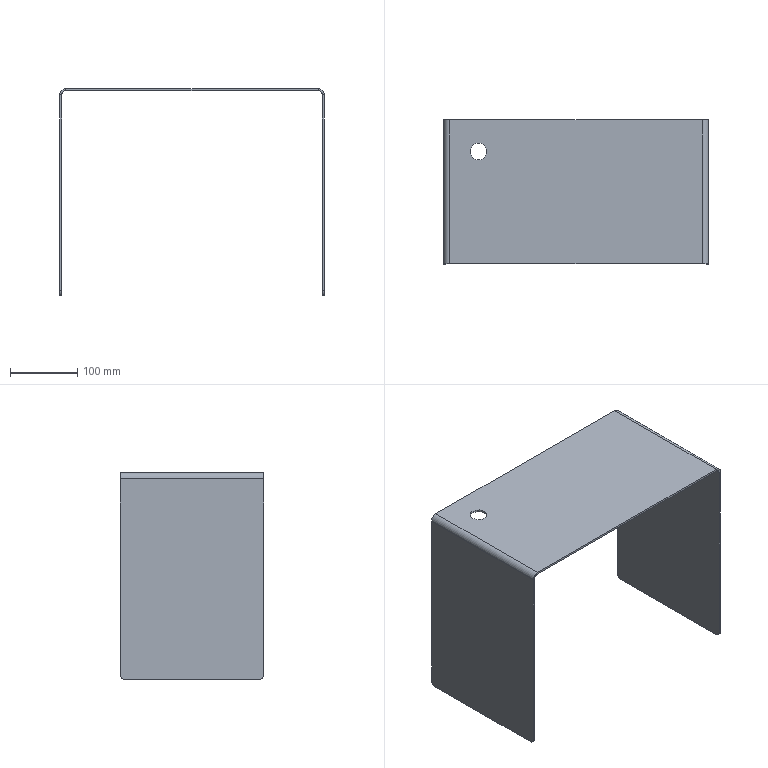Part | SolidWorks | features Fillet 1, FlatPattern 1, ICE 1, SMBaseFlange 1, SheetMetal 1 | 1 solid | 28 faces | box 394 x 214 x 307 mm | volume 637569 mm3 | plane 18 | cylinder 10 | commonest cylinder face diameters 13 x4 12 x2 18 x2 25 x2
STEP:
#1=CARTESIAN_POINT('',(64.5,167.,0.));
#2=VERTEX_POINT('',#1);
#3=CARTESIAN_POINT('',(39.5,167.,0.));
#4=VERTEX_POINT('',#3);
#5=CARTESIAN_POINT('',(52.,167.,0.));
#6=DIRECTION('',(0.,0.,-1.));
#7=DIRECTION('',(-1.,0.,0.));
#8=AXIS2_PLACEMENT_3D('',#5,#6,#7);
#9=CIRCLE('',#8,12.5);
#10=EDGE_CURVE('',#2,#4,#9,.T.);
#11=ORIENTED_EDGE('',*,*,#10,.F.);
#12=CARTESIAN_POINT('',(64.5,167.,-3.));
#13=VERTEX_POINT('',#12);
#14=CARTESIAN_POINT('',(64.5,167.,0.));
#15=DIRECTION('',(0.,0.,-1.));
#16=VECTOR('',#15,1000.);
#17=LINE('',#14,#16);
#18=EDGE_CURVE('',#2,#13,#17,.T.);
#19=ORIENTED_EDGE('',*,*,#18,.T.);
#20=CARTESIAN_POINT('',(39.5,167.,-3.));
#21=VERTEX_POINT('',#20);
#22=CARTESIAN_POINT('',(52.,167.,-3.));
#23=DIRECTION('',(0.,0.,-1.));
#24=DIRECTION('',(-1.,0.,0.));
#25=AXIS2_PLACEMENT_3D('',#22,#23,#24);
#26=CIRCLE('',#25,12.5);
#27=EDGE_CURVE('',#13,#21,#26,.T.);
#28=ORIENTED_EDGE('',*,*,#27,.T.);
#29=CARTESIAN_POINT('',(39.5,167.,0.));
#30=DIRECTION('',(0.,0.,-1.));
#31=VECTOR('',#30,1000.);
#32=LINE('',#29,#31);
#33=EDGE_CURVE('',#4,#21,#32,.T.);
#34=ORIENTED_EDGE('',*,*,#33,.F.);
#35=EDGE_LOOP('',(#11,#19,#28,#34));
#36=FACE_OUTER_BOUND('',#35,.T.);
#37=CARTESIAN_POINT('',(52.,167.,0.));
#38=DIRECTION('',(0.,0.,-1.));
#39=DIRECTION('',(-1.,0.,0.));
#40=AXIS2_PLACEMENT_3D('',#37,#38,#39);
#41=CYLINDRICAL_SURFACE('',#40,12.5);
#42=ADVANCED_FACE('',(#36),#41,.F.);
#43=CARTESIAN_POINT('',(0.,214.,-9.));
#44=VERTEX_POINT('',#43);
#45=CARTESIAN_POINT('',(3.,214.,-9.));
#46=VERTEX_POINT('',#45);
#47=CARTESIAN_POINT('',(0.,214.,-9.));
#48=DIRECTION('',(1.,0.,0.));
#49=VECTOR('',#48,1000.);
#50=LINE('',#47,#49);
#51=EDGE_CURVE('',#44,#46,#50,.T.);
#52=ORIENTED_EDGE('',*,*,#51,.F.);
#53=CARTESIAN_POINT('',(9.,214.,0.));
#54=VERTEX_POINT('',#53);
#55=CARTESIAN_POINT('',(9.,214.,-9.));
#56=DIRECTION('',(0.,1.,0.));
#57=DIRECTION('',(0.,0.,-1.));
#58=AXIS2_PLACEMENT_3D('',#55,#56,#57);
#59=CIRCLE('',#58,9.);
#60=EDGE_CURVE('',#44,#54,#59,.T.);
#61=ORIENTED_EDGE('',*,*,#60,.T.);
#62=CARTESIAN_POINT('',(9.,214.,-3.));
#63=VERTEX_POINT('',#62);
#64=CARTESIAN_POINT('',(9.,214.,-3.));
#65=DIRECTION('',(0.,0.,1.));
#66=VECTOR('',#65,1000.);
#67=LINE('',#64,#66);
#68=EDGE_CURVE('',#63,#54,#67,.T.);
#69=ORIENTED_EDGE('',*,*,#68,.F.);
#70=CARTESIAN_POINT('',(9.,214.,-9.));
#71=DIRECTION('',(0.,1.,0.));
#72=DIRECTION('',(1.,0.,0.));
#73=AXIS2_PLACEMENT_3D('',#70,#71,#72);
#74=CIRCLE('',#73,6.);
#75=EDGE_CURVE('',#46,#63,#74,.T.);
#76=ORIENTED_EDGE('',*,*,#75,.F.);
#77=EDGE_LOOP('',(#52,#61,#69,#76));
#78=FACE_OUTER_BOUND('',#77,.T.);
#79=CARTESIAN_POINT('',(0.,214.,-9.));
#80=DIRECTION('',(0.,1.,0.));
#81=DIRECTION('',(0.,0.,1.));
#82=AXIS2_PLACEMENT_3D('',#79,#80,#81);
#83=PLANE('',#82);
#84=ADVANCED_FACE('',(#78),#83,.T.);
#85=CARTESIAN_POINT('',(3.,214.,-300.5));
#86=VERTEX_POINT('',#85);
#87=CARTESIAN_POINT('',(3.,214.,0.));
#88=DIRECTION('',(0.,0.,1.));
#89=VECTOR('',#88,1000.);
#90=LINE('',#87,#89);
#91=EDGE_CURVE('',#86,#46,#90,.T.);
#92=ORIENTED_EDGE('',*,*,#91,.F.);
#93=CARTESIAN_POINT('',(0.,214.,-300.5));
#94=VERTEX_POINT('',#93);
#95=CARTESIAN_POINT('',(9.,214.,-300.5));
#96=DIRECTION('',(-1.,0.,0.));
#97=VECTOR('',#96,1000.);
#98=LINE('',#95,#97);
#99=EDGE_CURVE('',#86,#94,#98,.T.);
#100=ORIENTED_EDGE('',*,*,#99,.T.);
#101=CARTESIAN_POINT('',(0.,214.,0.));
#102=DIRECTION('',(0.,0.,1.));
#103=VECTOR('',#102,1000.);
#104=LINE('',#101,#103);
#105=EDGE_CURVE('',#94,#44,#104,.T.);
#106=ORIENTED_EDGE('',*,*,#105,.T.);
#107=ORIENTED_EDGE('',*,*,#51,.T.);
#108=EDGE_LOOP('',(#92,#100,#106,#107));
#109=FACE_OUTER_BOUND('',#108,.T.);
#110=CARTESIAN_POINT('',(9.,214.,-3.));
#111=DIRECTION('',(0.,1.,0.));
#112=DIRECTION('',(0.,0.,1.));
#113=AXIS2_PLACEMENT_3D('',#110,#111,#112);
#114=PLANE('',#113);
#115=ADVANCED_FACE('',(#109),#114,.T.);
#116=CARTESIAN_POINT('',(9.,0.,0.));
#117=VERTEX_POINT('',#116);
#118=CARTESIAN_POINT('',(9.,0.,-3.));
#119=VERTEX_POINT('',#118);
#120=CARTESIAN_POINT('',(9.,0.,0.));
#121=DIRECTION('',(0.,0.,-1.));
#122=VECTOR('',#121,1000.);
#123=LINE('',#120,#122);
#124=EDGE_CURVE('',#117,#119,#123,.T.);
#125=ORIENTED_EDGE('',*,*,#124,.F.);
#126=CARTESIAN_POINT('',(0.,0.,-9.));
#127=VERTEX_POINT('',#126);
#128=CARTESIAN_POINT('',(9.,0.,-9.));
#129=DIRECTION('',(0.,1.,0.));
#130=DIRECTION('',(0.,0.,-1.));
#131=AXIS2_PLACEMENT_3D('',#128,#129,#130);
#132=CIRCLE('',#131,9.);
#133=EDGE_CURVE('',#127,#117,#132,.T.);
#134=ORIENTED_EDGE('',*,*,#133,.F.);
#135=CARTESIAN_POINT('',(3.,0.,-9.));
#136=VERTEX_POINT('',#135);
#137=CARTESIAN_POINT('',(3.,0.,-9.));
#138=DIRECTION('',(-1.,0.,0.));
#139=VECTOR('',#138,1000.);
#140=LINE('',#137,#139);
#141=EDGE_CURVE('',#136,#127,#140,.T.);
#142=ORIENTED_EDGE('',*,*,#141,.F.);
#143=CARTESIAN_POINT('',(9.,0.,-9.));
#144=DIRECTION('',(0.,1.,0.));
#145=DIRECTION('',(1.,0.,0.));
#146=AXIS2_PLACEMENT_3D('',#143,#144,#145);
#147=CIRCLE('',#146,6.);
#148=EDGE_CURVE('',#136,#119,#147,.T.);
#149=ORIENTED_EDGE('',*,*,#148,.T.);
#150=EDGE_LOOP('',(#125,#134,#142,#149));
#151=FACE_OUTER_BOUND('',#150,.T.);
#152=CARTESIAN_POINT('',(9.,0.,0.));
#153=DIRECTION('',(0.,-1.,0.));
#154=DIRECTION('',(0.,0.,-1.));
#155=AXIS2_PLACEMENT_3D('',#152,#153,#154);
#156=PLANE('',#155);
#157=ADVANCED_FACE('',(#151),#156,.T.);
#158=CARTESIAN_POINT('',(385.,0.,0.));
#159=VERTEX_POINT('',#158);
#160=CARTESIAN_POINT('',(0.,0.,0.));
#161=DIRECTION('',(1.,0.,0.));
#162=VECTOR('',#161,1000.);
#163=LINE('',#160,#162);
#164=EDGE_CURVE('',#117,#159,#163,.T.);
#165=ORIENTED_EDGE('',*,*,#164,.F.);
#166=ORIENTED_EDGE('',*,*,#124,.T.);
#167=CARTESIAN_POINT('',(385.,0.,-3.));
#168=VERTEX_POINT('',#167);
#169=CARTESIAN_POINT('',(0.,0.,-3.));
#170=DIRECTION('',(1.,0.,0.));
#171=VECTOR('',#170,1000.);
#172=LINE('',#169,#171);
#173=EDGE_CURVE('',#119,#168,#172,.T.);
#174=ORIENTED_EDGE('',*,*,#173,.T.);
#175=CARTESIAN_POINT('',(385.,0.,-3.));
#176=DIRECTION('',(0.,0.,1.));
#177=VECTOR('',#176,1000.);
#178=LINE('',#175,#177);
#179=EDGE_CURVE('',#168,#159,#178,.T.);
#180=ORIENTED_EDGE('',*,*,#179,.T.);
#181=EDGE_LOOP('',(#165,#166,#174,#180));
#182=FACE_OUTER_BOUND('',#181,.T.);
#183=CARTESIAN_POINT('',(3.,0.,-9.));
#184=DIRECTION('',(0.,-1.,0.));
#185=DIRECTION('',(0.,0.,-1.));
#186=AXIS2_PLACEMENT_3D('',#183,#184,#185);
#187=PLANE('',#186);
#188=ADVANCED_FACE('',(#182),#187,.T.);
#189=CARTESIAN_POINT('',(385.,214.,0.));
#190=VERTEX_POINT('',#189);
#191=CARTESIAN_POINT('',(385.,214.,-3.));
#192=VERTEX_POINT('',#191);
#193=CARTESIAN_POINT('',(385.,214.,0.));
#194=DIRECTION('',(0.,0.,-1.));
#195=VECTOR('',#194,1000.);
#196=LINE('',#193,#195);
#197=EDGE_CURVE('',#190,#192,#196,.T.);
#198=ORIENTED_EDGE('',*,*,#197,.F.);
#199=CARTESIAN_POINT('',(394.,214.,-9.));
#200=VERTEX_POINT('',#199);
#201=CARTESIAN_POINT('',(385.,214.,-9.));
#202=DIRECTION('',(0.,1.,0.));
#203=DIRECTION('',(0.,0.,-1.));
#204=AXIS2_PLACEMENT_3D('',#201,#202,#203);
#205=CIRCLE('',#204,9.);
#206=EDGE_CURVE('',#190,#200,#205,.T.);
#207=ORIENTED_EDGE('',*,*,#206,.T.);
#208=CARTESIAN_POINT('',(391.,214.,-9.));
#209=VERTEX_POINT('',#208);
#210=CARTESIAN_POINT('',(391.,214.,-9.));
#211=DIRECTION('',(1.,0.,0.));
#212=VECTOR('',#211,1000.);
#213=LINE('',#210,#212);
#214=EDGE_CURVE('',#209,#200,#213,.T.);
#215=ORIENTED_EDGE('',*,*,#214,.F.);
#216=CARTESIAN_POINT('',(385.,214.,-9.));
#217=DIRECTION('',(0.,1.,0.));
#218=DIRECTION('',(1.,0.,0.));
#219=AXIS2_PLACEMENT_3D('',#216,#217,#218);
#220=CIRCLE('',#219,6.);
#221=EDGE_CURVE('',#192,#209,#220,.T.);
#222=ORIENTED_EDGE('',*,*,#221,.F.);
#223=EDGE_LOOP('',(#198,#207,#215,#222));
#224=FACE_OUTER_BOUND('',#223,.T.);
#225=CARTESIAN_POINT('',(385.,214.,0.));
#226=DIRECTION('',(0.,1.,0.));
#227=DIRECTION('',(0.,0.,1.));
#228=AXIS2_PLACEMENT_3D('',#225,#226,#227);
#229=PLANE('',#228);
#230=ADVANCED_FACE('',(#224),#229,.T.);
#231=CARTESIAN_POINT('',(0.,214.,0.));
#232=DIRECTION('',(1.,0.,0.));
#233=VECTOR('',#232,1000.);
#234=LINE('',#231,#233);
#235=EDGE_CURVE('',#54,#190,#234,.T.);
#236=ORIENTED_EDGE('',*,*,#235,.T.);
#237=ORIENTED_EDGE('',*,*,#197,.T.);
#238=CARTESIAN_POINT('',(0.,214.,-3.));
#239=DIRECTION('',(1.,0.,0.));
#240=VECTOR('',#239,1000.);
#241=LINE('',#238,#240);
#242=EDGE_CURVE('',#63,#192,#241,.T.);
#243=ORIENTED_EDGE('',*,*,#242,.F.);
#244=ORIENTED_EDGE('',*,*,#68,.T.);
#245=EDGE_LOOP('',(#236,#237,#243,#244));
#246=FACE_OUTER_BOUND('',#245,.T.);
#247=CARTESIAN_POINT('',(391.,214.,-9.));
#248=DIRECTION('',(0.,1.,0.));
#249=DIRECTION('',(0.,0.,1.));
#250=AXIS2_PLACEMENT_3D('',#247,#248,#249);
#251=PLANE('',#250);
#252=ADVANCED_FACE('',(#246),#251,.T.);
#253=CARTESIAN_POINT('',(394.,0.,-9.));
#254=VERTEX_POINT('',#253);
#255=CARTESIAN_POINT('',(391.,0.,-9.));
#256=VERTEX_POINT('',#255);
#257=CARTESIAN_POINT('',(394.,0.,-9.));
#258=DIRECTION('',(-1.,0.,0.));
#259=VECTOR('',#258,1000.);
#260=LINE('',#257,#259);
#261=EDGE_CURVE('',#254,#256,#260,.T.);
#262=ORIENTED_EDGE('',*,*,#261,.F.);
#263=CARTESIAN_POINT('',(385.,0.,-9.));
#264=DIRECTION('',(0.,1.,0.));
#265=DIRECTION('',(0.,0.,-1.));
#266=AXIS2_PLACEMENT_3D('',#263,#264,#265);
#267=CIRCLE('',#266,9.);
#268=EDGE_CURVE('',#159,#254,#267,.T.);
#269=ORIENTED_EDGE('',*,*,#268,.F.);
#270=ORIENTED_EDGE('',*,*,#179,.F.);
#271=CARTESIAN_POINT('',(385.,0.,-9.));
#272=DIRECTION('',(0.,1.,0.));
#273=DIRECTION('',(1.,0.,0.));
#274=AXIS2_PLACEMENT_3D('',#271,#272,#273);
#275=CIRCLE('',#274,6.);
#276=EDGE_CURVE('',#168,#256,#275,.T.);
#277=ORIENTED_EDGE('',*,*,#276,.T.);
#278=EDGE_LOOP('',(#262,#269,#270,#277));
#279=FACE_OUTER_BOUND('',#278,.T.);
#280=CARTESIAN_POINT('',(394.,0.,-9.));
#281=DIRECTION('',(0.,-1.,0.));
#282=DIRECTION('',(0.,0.,-1.));
#283=AXIS2_PLACEMENT_3D('',#280,#281,#282);
#284=PLANE('',#283);
#285=ADVANCED_FACE('',(#279),#284,.T.);
#286=CARTESIAN_POINT('',(391.,0.,-300.5));
#287=VERTEX_POINT('',#286);
#288=CARTESIAN_POINT('',(391.,0.,0.));
#289=DIRECTION('',(0.,0.,-1.));
#290=VECTOR('',#289,1000.);
#291=LINE('',#288,#290);
#292=EDGE_CURVE('',#256,#287,#291,.T.);
#293=ORIENTED_EDGE('',*,*,#292,.T.);
#294=CARTESIAN_POINT('',(394.,0.,-300.5));
#295=VERTEX_POINT('',#294);
#296=CARTESIAN_POINT('',(385.,0.,-300.5));
#297=DIRECTION('',(1.,0.,0.));
#298=VECTOR('',#297,1000.);
#299=LINE('',#296,#298);
#300=EDGE_CURVE('',#287,#295,#299,.T.);
#301=ORIENTED_EDGE('',*,*,#300,.T.);
#302=CARTESIAN_POINT('',(394.,0.,0.));
#303=DIRECTION('',(0.,0.,-1.));
#304=VECTOR('',#303,1000.);
#305=LINE('',#302,#304);
#306=EDGE_CURVE('',#254,#295,#305,.T.);
#307=ORIENTED_EDGE('',*,*,#306,.F.);
#308=ORIENTED_EDGE('',*,*,#261,.T.);
#309=EDGE_LOOP('',(#293,#301,#307,#308));
#310=FACE_OUTER_BOUND('',#309,.T.);
#311=CARTESIAN_POINT('',(385.,0.,-3.));
#312=DIRECTION('',(0.,-1.,0.));
#313=DIRECTION('',(0.,0.,-1.));
#314=AXIS2_PLACEMENT_3D('',#311,#312,#313);
#315=PLANE('',#314);
#316=ADVANCED_FACE('',(#310),#315,.T.);
#317=ORIENTED_EDGE('',*,*,#306,.T.);
#318=CARTESIAN_POINT('',(394.,6.5,-307.));
#319=VERTEX_POINT('',#318);
#320=CARTESIAN_POINT('',(394.,6.5,-300.5));
#321=DIRECTION('',(1.,0.,0.));
#322=DIRECTION('',(0.,0.,1.));
#323=AXIS2_PLACEMENT_3D('',#320,#321,#322);
#324=CIRCLE('',#323,6.5);
#325=EDGE_CURVE('',#295,#319,#324,.T.);
#326=ORIENTED_EDGE('',*,*,#325,.T.);
#327=CARTESIAN_POINT('',(394.,207.5,-307.));
#328=VERTEX_POINT('',#327);
#329=CARTESIAN_POINT('',(394.,214.,-307.));
#330=DIRECTION('',(0.,-1.,0.));
#331=VECTOR('',#330,1000.);
#332=LINE('',#329,#331);
#333=EDGE_CURVE('',#328,#319,#332,.T.);
#334=ORIENTED_EDGE('',*,*,#333,.F.);
#335=CARTESIAN_POINT('',(394.,214.,-300.5));
#336=VERTEX_POINT('',#335);
#337=CARTESIAN_POINT('',(394.,207.5,-300.5));
#338=DIRECTION('',(1.,0.,0.));
#339=DIRECTION('',(0.,0.,1.));
#340=AXIS2_PLACEMENT_3D('',#337,#338,#339);
#341=CIRCLE('',#340,6.5);
#342=EDGE_CURVE('',#328,#336,#341,.T.);
#343=ORIENTED_EDGE('',*,*,#342,.T.);
#344=CARTESIAN_POINT('',(394.,214.,0.));
#345=DIRECTION('',(0.,0.,-1.));
#346=VECTOR('',#345,1000.);
#347=LINE('',#344,#346);
#348=EDGE_CURVE('',#200,#336,#347,.T.);
#349=ORIENTED_EDGE('',*,*,#348,.F.);
#350=CARTESIAN_POINT('',(394.,214.,-9.));
#351=DIRECTION('',(0.,-1.,0.));
#352=VECTOR('',#351,1000.);
#353=LINE('',#350,#352);
#354=EDGE_CURVE('',#200,#254,#353,.T.);
#355=ORIENTED_EDGE('',*,*,#354,.T.);
#356=EDGE_LOOP('',(#317,#326,#334,#343,#349,#355));
#357=FACE_OUTER_BOUND('',#356,.T.);
#358=CARTESIAN_POINT('',(394.,214.,0.));
#359=DIRECTION('',(-1.,0.,0.));
#360=DIRECTION('',(0.,0.,1.));
#361=AXIS2_PLACEMENT_3D('',#358,#359,#360);
#362=PLANE('',#361);
#363=ADVANCED_FACE('',(#357),#362,.F.);
#364=ORIENTED_EDGE('',*,*,#333,.T.);
#365=CARTESIAN_POINT('',(391.,6.5,-307.));
#366=VERTEX_POINT('',#365);
#367=CARTESIAN_POINT('',(391.,6.5,-307.));
#368=DIRECTION('',(-1.,0.,0.));
#369=VECTOR('',#368,1000.);
#370=LINE('',#367,#369);
#371=EDGE_CURVE('',#319,#366,#370,.T.);
#372=ORIENTED_EDGE('',*,*,#371,.T.);
#373=CARTESIAN_POINT('',(391.,207.5,-307.));
#374=VERTEX_POINT('',#373);
#375=CARTESIAN_POINT('',(391.,214.,-307.));
#376=DIRECTION('',(0.,-1.,0.));
#377=VECTOR('',#376,1000.);
#378=LINE('',#375,#377);
#379=EDGE_CURVE('',#374,#366,#378,.T.);
#380=ORIENTED_EDGE('',*,*,#379,.F.);
#381=CARTESIAN_POINT('',(391.,207.5,-307.));
#382=DIRECTION('',(1.,0.,0.));
#383=VECTOR('',#382,1000.);
#384=LINE('',#381,#383);
#385=EDGE_CURVE('',#374,#328,#384,.T.);
#386=ORIENTED_EDGE('',*,*,#385,.T.);
#387=EDGE_LOOP('',(#364,#372,#380,#386));
#388=FACE_OUTER_BOUND('',#387,.T.);
#389=CARTESIAN_POINT('',(391.,214.,-307.));
#390=DIRECTION('',(0.,0.,-1.));
#391=DIRECTION('',(-1.,0.,0.));
#392=AXIS2_PLACEMENT_3D('',#389,#390,#391);
#393=PLANE('',#392);
#394=ADVANCED_FACE('',(#388),#393,.T.);
#395=ORIENTED_EDGE('',*,*,#379,.T.);
#396=CARTESIAN_POINT('',(391.,6.5,-300.5));
#397=DIRECTION('',(-1.,0.,0.));
#398=DIRECTION('',(0.,0.,1.));
#399=AXIS2_PLACEMENT_3D('',#396,#397,#398);
#400=CIRCLE('',#399,6.5);
#401=EDGE_CURVE('',#366,#287,#400,.T.);
#402=ORIENTED_EDGE('',*,*,#401,.T.);
#403=ORIENTED_EDGE('',*,*,#292,.F.);
#404=CARTESIAN_POINT('',(391.,214.,-9.));
#405=DIRECTION('',(0.,-1.,0.));
#406=VECTOR('',#405,1000.);
#407=LINE('',#404,#406);
#408=EDGE_CURVE('',#209,#256,#407,.T.);
#409=ORIENTED_EDGE('',*,*,#408,.F.);
#410=CARTESIAN_POINT('',(391.,214.,-300.5));
#411=VERTEX_POINT('',#410);
#412=CARTESIAN_POINT('',(391.,214.,0.));
#413=DIRECTION('',(0.,0.,-1.));
#414=VECTOR('',#413,1000.);
#415=LINE('',#412,#414);
#416=EDGE_CURVE('',#209,#411,#415,.T.);
#417=ORIENTED_EDGE('',*,*,#416,.T.);
#418=CARTESIAN_POINT('',(391.,207.5,-300.5));
#419=DIRECTION('',(-1.,0.,0.));
#420=DIRECTION('',(0.,0.,1.));
#421=AXIS2_PLACEMENT_3D('',#418,#419,#420);
#422=CIRCLE('',#421,6.5);
#423=EDGE_CURVE('',#411,#374,#422,.T.);
#424=ORIENTED_EDGE('',*,*,#423,.T.);
#425=EDGE_LOOP('',(#395,#402,#403,#409,#417,#424));
#426=FACE_OUTER_BOUND('',#425,.T.);
#427=CARTESIAN_POINT('',(391.,214.,0.));
#428=DIRECTION('',(-1.,0.,0.));
#429=DIRECTION('',(0.,0.,1.));
#430=AXIS2_PLACEMENT_3D('',#427,#428,#429);
#431=PLANE('',#430);
#432=ADVANCED_FACE('',(#426),#431,.T.);
#433=ORIENTED_EDGE('',*,*,#276,.F.);
#434=CARTESIAN_POINT('',(385.,214.,-3.));
#435=DIRECTION('',(0.,-1.,0.));
#436=VECTOR('',#435,1000.);
#437=LINE('',#434,#436);
#438=EDGE_CURVE('',#192,#168,#437,.T.);
#439=ORIENTED_EDGE('',*,*,#438,.F.);
#440=ORIENTED_EDGE('',*,*,#221,.T.);
#441=ORIENTED_EDGE('',*,*,#408,.T.);
#442=EDGE_LOOP('',(#433,#439,#440,#441));
#443=FACE_OUTER_BOUND('',#442,.T.);
#444=CARTESIAN_POINT('',(385.,214.,-9.));
#445=DIRECTION('',(0.,-1.,0.));
#446=DIRECTION('',(0.,0.,-1.));
#447=AXIS2_PLACEMENT_3D('',#444,#445,#446);
#448=CYLINDRICAL_SURFACE('',#447,6.);
#449=ADVANCED_FACE('',(#443),#448,.F.);
#450=CARTESIAN_POINT('',(52.,167.,-3.));
#451=DIRECTION('',(0.,0.,-1.));
#452=DIRECTION('',(-1.,0.,0.));
#453=AXIS2_PLACEMENT_3D('',#450,#451,#452);
#454=CIRCLE('',#453,12.5);
#455=EDGE_CURVE('',#21,#13,#454,.T.);
#456=ORIENTED_EDGE('',*,*,#455,.F.);
#457=ORIENTED_EDGE('',*,*,#27,.F.);
#458=EDGE_LOOP('',(#456,#457));
#459=FACE_BOUND('',#458,.T.);
#460=ORIENTED_EDGE('',*,*,#173,.F.);
#461=CARTESIAN_POINT('',(9.,214.,-3.));
#462=DIRECTION('',(0.,-1.,0.));
#463=VECTOR('',#462,1000.);
#464=LINE('',#461,#463);
#465=EDGE_CURVE('',#63,#119,#464,.T.);
#466=ORIENTED_EDGE('',*,*,#465,.F.);
#467=ORIENTED_EDGE('',*,*,#242,.T.);
#468=ORIENTED_EDGE('',*,*,#438,.T.);
#469=EDGE_LOOP('',(#460,#466,#467,#468));
#470=FACE_OUTER_BOUND('',#469,.T.);
#471=CARTESIAN_POINT('',(0.,214.,-3.));
#472=DIRECTION('',(0.,0.,-1.));
#473=DIRECTION('',(-1.,0.,0.));
#474=AXIS2_PLACEMENT_3D('',#471,#472,#473);
#475=PLANE('',#474);
#476=ADVANCED_FACE('',(#459,#470),#475,.T.);
#477=ORIENTED_EDGE('',*,*,#148,.F.);
#478=CARTESIAN_POINT('',(3.,214.,-9.));
#479=DIRECTION('',(0.,-1.,0.));
#480=VECTOR('',#479,1000.);
#481=LINE('',#478,#480);
#482=EDGE_CURVE('',#46,#136,#481,.T.);
#483=ORIENTED_EDGE('',*,*,#482,.F.);
#484=ORIENTED_EDGE('',*,*,#75,.T.);
#485=ORIENTED_EDGE('',*,*,#465,.T.);
#486=EDGE_LOOP('',(#477,#483,#484,#485));
#487=FACE_OUTER_BOUND('',#486,.T.);
#488=CARTESIAN_POINT('',(9.,214.,-9.));
#489=DIRECTION('',(0.,-1.,0.));
#490=DIRECTION('',(0.,0.,-1.));
#491=AXIS2_PLACEMENT_3D('',#488,#489,#490);
#492=CYLINDRICAL_SURFACE('',#491,6.);
#493=ADVANCED_FACE('',(#487),#492,.F.);
#494=CARTESIAN_POINT('',(3.,0.,-300.5));
#495=VERTEX_POINT('',#494);
#496=CARTESIAN_POINT('',(3.,0.,0.));
#497=DIRECTION('',(0.,0.,1.));
#498=VECTOR('',#497,1000.);
#499=LINE('',#496,#498);
#500=EDGE_CURVE('',#495,#136,#499,.T.);
#501=ORIENTED_EDGE('',*,*,#500,.F.);
#502=CARTESIAN_POINT('',(3.,6.5,-307.));
#503=VERTEX_POINT('',#502);
#504=CARTESIAN_POINT('',(3.,6.5,-300.5));
#505=DIRECTION('',(1.,0.,0.));
#506=DIRECTION('',(0.,0.,-1.));
#507=AXIS2_PLACEMENT_3D('',#504,#505,#506);
#508=CIRCLE('',#507,6.5);
#509=EDGE_CURVE('',#495,#503,#508,.T.);
#510=ORIENTED_EDGE('',*,*,#509,.T.);
#511=CARTESIAN_POINT('',(3.,207.5,-307.));
#512=VERTEX_POINT('',#511);
#513=CARTESIAN_POINT('',(3.,214.,-307.));
#514=DIRECTION('',(0.,-1.,0.));
#515=VECTOR('',#514,1000.);
#516=LINE('',#513,#515);
#517=EDGE_CURVE('',#512,#503,#516,.T.);
#518=ORIENTED_EDGE('',*,*,#517,.F.);
#519=CARTESIAN_POINT('',(3.,207.5,-300.5));
#520=DIRECTION('',(1.,0.,0.));
#521=DIRECTION('',(0.,0.,-1.));
#522=AXIS2_PLACEMENT_3D('',#519,#520,#521);
#523=CIRCLE('',#522,6.5);
#524=EDGE_CURVE('',#512,#86,#523,.T.);
#525=ORIENTED_EDGE('',*,*,#524,.T.);
#526=ORIENTED_EDGE('',*,*,#91,.T.);
#527=ORIENTED_EDGE('',*,*,#482,.T.);
#528=EDGE_LOOP('',(#501,#510,#518,#525,#526,#527));
#529=FACE_OUTER_BOUND('',#528,.T.);
#530=CARTESIAN_POINT('',(3.,214.,0.));
#531=DIRECTION('',(1.,0.,0.));
#532=DIRECTION('',(0.,0.,-1.));
#533=AXIS2_PLACEMENT_3D('',#530,#531,#532);
#534=PLANE('',#533);
#535=ADVANCED_FACE('',(#529),#534,.T.);
#536=ORIENTED_EDGE('',*,*,#517,.T.);
#537=CARTESIAN_POINT('',(0.,6.5,-307.));
#538=VERTEX_POINT('',#537);
#539=CARTESIAN_POINT('',(0.,6.5,-307.));
#540=DIRECTION('',(-1.,0.,0.));
#541=VECTOR('',#540,1000.);
#542=LINE('',#539,#541);
#543=EDGE_CURVE('',#503,#538,#542,.T.);
#544=ORIENTED_EDGE('',*,*,#543,.T.);
#545=CARTESIAN_POINT('',(0.,207.5,-307.));
#546=VERTEX_POINT('',#545);
#547=CARTESIAN_POINT('',(0.,214.,-307.));
#548=DIRECTION('',(0.,-1.,0.));
#549=VECTOR('',#548,1000.);
#550=LINE('',#547,#549);
#551=EDGE_CURVE('',#546,#538,#550,.T.);
#552=ORIENTED_EDGE('',*,*,#551,.F.);
#553=CARTESIAN_POINT('',(0.,207.5,-307.));
#554=DIRECTION('',(1.,0.,0.));
#555=VECTOR('',#554,1000.);
#556=LINE('',#553,#555);
#557=EDGE_CURVE('',#546,#512,#556,.T.);
#558=ORIENTED_EDGE('',*,*,#557,.T.);
#559=EDGE_LOOP('',(#536,#544,#552,#558));
#560=FACE_OUTER_BOUND('',#559,.T.);
#561=CARTESIAN_POINT('',(0.,214.,-307.));
#562=DIRECTION('',(0.,0.,-1.));
#563=DIRECTION('',(-1.,0.,0.));
#564=AXIS2_PLACEMENT_3D('',#561,#562,#563);
#565=PLANE('',#564);
#566=ADVANCED_FACE('',(#560),#565,.T.);
#567=ORIENTED_EDGE('',*,*,#551,.T.);
#568=CARTESIAN_POINT('',(0.,0.,-300.5));
#569=VERTEX_POINT('',#568);
#570=CARTESIAN_POINT('',(0.,6.5,-300.5));
#571=DIRECTION('',(-1.,0.,0.));
#572=DIRECTION('',(0.,0.,-1.));
#573=AXIS2_PLACEMENT_3D('',#570,#571,#572);
#574=CIRCLE('',#573,6.5);
#575=EDGE_CURVE('',#538,#569,#574,.T.);
#576=ORIENTED_EDGE('',*,*,#575,.T.);
#577=CARTESIAN_POINT('',(0.,0.,0.));
#578=DIRECTION('',(0.,0.,1.));
#579=VECTOR('',#578,1000.);
#580=LINE('',#577,#579);
#581=EDGE_CURVE('',#569,#127,#580,.T.);
#582=ORIENTED_EDGE('',*,*,#581,.T.);
#583=CARTESIAN_POINT('',(0.,214.,-9.));
#584=DIRECTION('',(0.,-1.,0.));
#585=VECTOR('',#584,1000.);
#586=LINE('',#583,#585);
#587=EDGE_CURVE('',#44,#127,#586,.T.);
#588=ORIENTED_EDGE('',*,*,#587,.F.);
#589=ORIENTED_EDGE('',*,*,#105,.F.);
#590=CARTESIAN_POINT('',(0.,207.5,-300.5));
#591=DIRECTION('',(-1.,0.,0.));
#592=DIRECTION('',(0.,0.,-1.));
#593=AXIS2_PLACEMENT_3D('',#590,#591,#592);
#594=CIRCLE('',#593,6.5);
#595=EDGE_CURVE('',#94,#546,#594,.T.);
#596=ORIENTED_EDGE('',*,*,#595,.T.);
#597=EDGE_LOOP('',(#567,#576,#582,#588,#589,#596));
#598=FACE_OUTER_BOUND('',#597,.T.);
#599=CARTESIAN_POINT('',(0.,214.,0.));
#600=DIRECTION('',(1.,0.,0.));
#601=DIRECTION('',(0.,0.,-1.));
#602=AXIS2_PLACEMENT_3D('',#599,#600,#601);
#603=PLANE('',#602);
#604=ADVANCED_FACE('',(#598),#603,.F.);
#605=ORIENTED_EDGE('',*,*,#133,.T.);
#606=CARTESIAN_POINT('',(9.,214.,0.));
#607=DIRECTION('',(0.,-1.,0.));
#608=VECTOR('',#607,1000.);
#609=LINE('',#606,#608);
#610=EDGE_CURVE('',#54,#117,#609,.T.);
#611=ORIENTED_EDGE('',*,*,#610,.F.);
#612=ORIENTED_EDGE('',*,*,#60,.F.);
#613=ORIENTED_EDGE('',*,*,#587,.T.);
#614=EDGE_LOOP('',(#605,#611,#612,#613));
#615=FACE_OUTER_BOUND('',#614,.T.);
#616=CARTESIAN_POINT('',(9.,214.,-9.));
#617=DIRECTION('',(0.,-1.,0.));
#618=DIRECTION('',(0.,0.,-1.));
#619=AXIS2_PLACEMENT_3D('',#616,#617,#618);
#620=CYLINDRICAL_SURFACE('',#619,9.);
#621=ADVANCED_FACE('',(#615),#620,.T.);
#622=CARTESIAN_POINT('',(52.,167.,0.));
#623=DIRECTION('',(0.,0.,-1.));
#624=DIRECTION('',(-1.,0.,0.));
#625=AXIS2_PLACEMENT_3D('',#622,#623,#624);
#626=CIRCLE('',#625,12.5);
#627=EDGE_CURVE('',#4,#2,#626,.T.);
#628=ORIENTED_EDGE('',*,*,#627,.T.);
#629=ORIENTED_EDGE('',*,*,#10,.T.);
#630=EDGE_LOOP('',(#628,#629));
#631=FACE_BOUND('',#630,.T.);
#632=ORIENTED_EDGE('',*,*,#164,.T.);
#633=CARTESIAN_POINT('',(385.,214.,0.));
#634=DIRECTION('',(0.,-1.,0.));
#635=VECTOR('',#634,1000.);
#636=LINE('',#633,#635);
#637=EDGE_CURVE('',#190,#159,#636,.T.);
#638=ORIENTED_EDGE('',*,*,#637,.F.);
#639=ORIENTED_EDGE('',*,*,#235,.F.);
#640=ORIENTED_EDGE('',*,*,#610,.T.);
#641=EDGE_LOOP('',(#632,#638,#639,#640));
#642=FACE_OUTER_BOUND('',#641,.T.);
#643=CARTESIAN_POINT('',(0.,214.,0.));
#644=DIRECTION('',(0.,0.,-1.));
#645=DIRECTION('',(-1.,0.,0.));
#646=AXIS2_PLACEMENT_3D('',#643,#644,#645);
#647=PLANE('',#646);
#648=ADVANCED_FACE('',(#631,#642),#647,.F.);
#649=ORIENTED_EDGE('',*,*,#268,.T.);
#650=ORIENTED_EDGE('',*,*,#354,.F.);
#651=ORIENTED_EDGE('',*,*,#206,.F.);
#652=ORIENTED_EDGE('',*,*,#637,.T.);
#653=EDGE_LOOP('',(#649,#650,#651,#652));
#654=FACE_OUTER_BOUND('',#653,.T.);
#655=CARTESIAN_POINT('',(385.,214.,-9.));
#656=DIRECTION('',(0.,-1.,0.));
#657=DIRECTION('',(0.,0.,-1.));
#658=AXIS2_PLACEMENT_3D('',#655,#656,#657);
#659=CYLINDRICAL_SURFACE('',#658,9.);
#660=ADVANCED_FACE('',(#654),#659,.T.);
#661=ORIENTED_EDGE('',*,*,#348,.T.);
#662=CARTESIAN_POINT('',(385.,214.,-300.5));
#663=DIRECTION('',(-1.,0.,0.));
#664=VECTOR('',#663,1000.);
#665=LINE('',#662,#664);
#666=EDGE_CURVE('',#336,#411,#665,.T.);
#667=ORIENTED_EDGE('',*,*,#666,.T.);
#668=ORIENTED_EDGE('',*,*,#416,.F.);
#669=ORIENTED_EDGE('',*,*,#214,.T.);
#670=EDGE_LOOP('',(#661,#667,#668,#669));
#671=FACE_OUTER_BOUND('',#670,.T.);
#672=CARTESIAN_POINT('',(385.,214.,-9.));
#673=DIRECTION('',(0.,1.,0.));
#674=DIRECTION('',(1.,0.,0.));
#675=AXIS2_PLACEMENT_3D('',#672,#673,#674);
#676=PLANE('',#675);
#677=ADVANCED_FACE('',(#671),#676,.T.);
#678=ORIENTED_EDGE('',*,*,#581,.F.);
#679=CARTESIAN_POINT('',(3.,0.,-300.5));
#680=DIRECTION('',(1.,0.,0.));
#681=VECTOR('',#680,1000.);
#682=LINE('',#679,#681);
#683=EDGE_CURVE('',#569,#495,#682,.T.);
#684=ORIENTED_EDGE('',*,*,#683,.T.);
#685=ORIENTED_EDGE('',*,*,#500,.T.);
#686=ORIENTED_EDGE('',*,*,#141,.T.);
#687=EDGE_LOOP('',(#678,#684,#685,#686));
#688=FACE_OUTER_BOUND('',#687,.T.);
#689=CARTESIAN_POINT('',(385.,0.,-9.));
#690=DIRECTION('',(0.,1.,0.));
#691=DIRECTION('',(1.,0.,0.));
#692=AXIS2_PLACEMENT_3D('',#689,#690,#691);
#693=PLANE('',#692);
#694=ADVANCED_FACE('',(#688),#693,.F.);
#695=ORIENTED_EDGE('',*,*,#18,.F.);
#696=ORIENTED_EDGE('',*,*,#627,.F.);
#697=ORIENTED_EDGE('',*,*,#33,.T.);
#698=ORIENTED_EDGE('',*,*,#455,.T.);
#699=EDGE_LOOP('',(#695,#696,#697,#698));
#700=FACE_OUTER_BOUND('',#699,.T.);
#701=CARTESIAN_POINT('',(52.,167.,0.));
#702=DIRECTION('',(0.,0.,-1.));
#703=DIRECTION('',(-1.,0.,0.));
#704=AXIS2_PLACEMENT_3D('',#701,#702,#703);
#705=CYLINDRICAL_SURFACE('',#704,12.5);
#706=ADVANCED_FACE('',(#700),#705,.F.);
#707=ORIENTED_EDGE('',*,*,#575,.F.);
#708=ORIENTED_EDGE('',*,*,#543,.F.);
#709=ORIENTED_EDGE('',*,*,#509,.F.);
#710=ORIENTED_EDGE('',*,*,#683,.F.);
#711=EDGE_LOOP('',(#707,#708,#709,#710));
#712=FACE_OUTER_BOUND('',#711,.T.);
#713=CARTESIAN_POINT('',(385.,6.5,-300.5));
#714=DIRECTION('',(-1.,0.,0.));
#715=DIRECTION('',(0.,0.,1.));
#716=AXIS2_PLACEMENT_3D('',#713,#714,#715);
#717=CYLINDRICAL_SURFACE('',#716,6.5);
#718=ADVANCED_FACE('',(#712),#717,.T.);
#719=ORIENTED_EDGE('',*,*,#401,.F.);
#720=ORIENTED_EDGE('',*,*,#371,.F.);
#721=ORIENTED_EDGE('',*,*,#325,.F.);
#722=ORIENTED_EDGE('',*,*,#300,.F.);
#723=EDGE_LOOP('',(#719,#720,#721,#722));
#724=FACE_OUTER_BOUND('',#723,.T.);
#725=CARTESIAN_POINT('',(385.,6.5,-300.5));
#726=DIRECTION('',(1.,0.,0.));
#727=DIRECTION('',(0.,0.,-1.));
#728=AXIS2_PLACEMENT_3D('',#725,#726,#727);
#729=CYLINDRICAL_SURFACE('',#728,6.5);
#730=ADVANCED_FACE('',(#724),#729,.T.);
#731=ORIENTED_EDGE('',*,*,#595,.F.);
#732=ORIENTED_EDGE('',*,*,#99,.F.);
#733=ORIENTED_EDGE('',*,*,#524,.F.);
#734=ORIENTED_EDGE('',*,*,#557,.F.);
#735=EDGE_LOOP('',(#731,#732,#733,#734));
#736=FACE_OUTER_BOUND('',#735,.T.);
#737=CARTESIAN_POINT('',(0.,207.5,-300.5));
#738=DIRECTION('',(1.,0.,0.));
#739=DIRECTION('',(0.,0.,-1.));
#740=AXIS2_PLACEMENT_3D('',#737,#738,#739);
#741=CYLINDRICAL_SURFACE('',#740,6.5);
#742=ADVANCED_FACE('',(#736),#741,.T.);
#743=ORIENTED_EDGE('',*,*,#423,.F.);
#744=ORIENTED_EDGE('',*,*,#666,.F.);
#745=ORIENTED_EDGE('',*,*,#342,.F.);
#746=ORIENTED_EDGE('',*,*,#385,.F.);
#747=EDGE_LOOP('',(#743,#744,#745,#746));
#748=FACE_OUTER_BOUND('',#747,.T.);
#749=CARTESIAN_POINT('',(391.,207.5,-300.5));
#750=DIRECTION('',(1.,0.,0.));
#751=DIRECTION('',(0.,0.,-1.));
#752=AXIS2_PLACEMENT_3D('',#749,#750,#751);
#753=CYLINDRICAL_SURFACE('',#752,6.5);
#754=ADVANCED_FACE('',(#748),#753,.T.);
#755=CLOSED_SHELL('',(#42,#84,#115,#157,#188,#230,#252,#285,#316,#363,#394,#432,#449,#476,#493,#535,#566,#604,#621,#648,#660,#677,#694,#706,#718,#730,#742,#754));
#756=MANIFOLD_SOLID_BREP('',#755);
#757=CARTESIAN_POINT('',(0.,0.,0.));
#758=DIRECTION('',(0.,0.,1.));
#759=DIRECTION('',(1.,0.,0.));
#760=AXIS2_PLACEMENT_3D('',#757,#758,#759);
#761=(LENGTH_UNIT()NAMED_UNIT(*)SI_UNIT(.MILLI.,.METRE.));
#762=UNCERTAINTY_MEASURE_WITH_UNIT(LENGTH_MEASURE(0.00001),#761,'','');
#763=(NAMED_UNIT(*)PLANE_ANGLE_UNIT()SI_UNIT($,.RADIAN.));
#764=(NAMED_UNIT(*)SI_UNIT($,.STERADIAN.)SOLID_ANGLE_UNIT());
#765=(GEOMETRIC_REPRESENTATION_CONTEXT(3)GLOBAL_UNCERTAINTY_ASSIGNED_CONTEXT((#762))GLOBAL_UNIT_ASSIGNED_CONTEXT((#761,#763,#764))REPRESENTATION_CONTEXT('',''));
#766=ADVANCED_BREP_SHAPE_REPRESENTATION('',(#756,#760),#765);